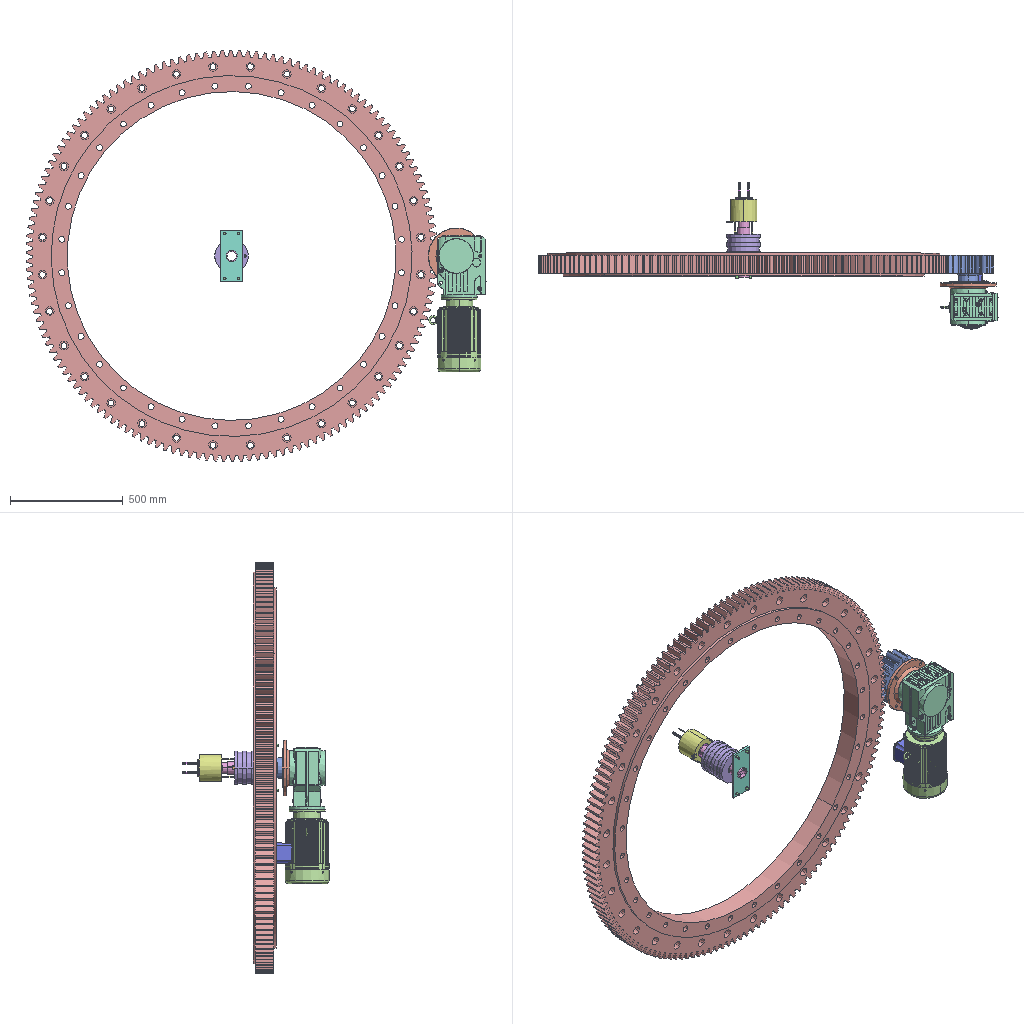Assembly | SolidWorks | 12 different items | 21 placed | box 2040 x 648 x 1824 mm
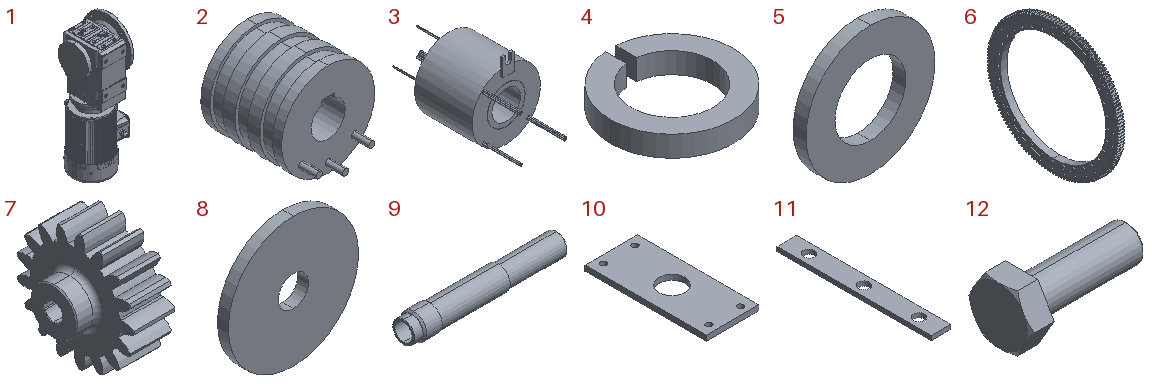Parts list (item | name | quantity | size | volume | features):
1 | (subassembly) | x1 | 274.5 x 257 x 638 mm | 13749904 mm3 | -
2 | - | x1 | 150 x 158 x 150 mm | 1845061 mm3 | features ICE 2, Revolution 1
3 | - | x1 | 119 x 236.5 x 137.5 mm | 931913 mm3 | features MBimport 1
4 | - | x4 | 15.372 x 15.344 x 2.6 mm | 261.313 mm3 | features Extrusion 1
5 | - | x4 | 20 x 2 x 20 mm | 438.252 mm3 | features Revolution 1
6 | - | x1 | 102 x 1824 x 1824 mm | 72400415 mm3 | features ICE 4, SketchHole 4, CirPattern 1, Stock 1
7 | - | x1 | 122 x 226.585 x 227.513 mm | 2321218 mm3 | features Chamfer 4, ICE 2, Fillet 1, MoveFace 1, SketchHole 1, Stock 1
8 | - | x1 | 60 x 5 x 60 mm | 13367 mm3 | features Extrusion 1
9 | - | x1 | 355 x 60 x 60 mm | 349894 mm3 | features Chamfer 1, Fillet 1, Revolution 1
10 | - | x1 | 100 x 230 x 10 mm | 206564 mm3 | features Extrusion 1
11 | - | x1 | 18 x 140 x 4 mm | 9138 mm3 | features Extrusion 1
12 | - | x4 | 36.4 x 18.475 x 16 mm | 3775 mm3 | features Chamfer 2, RevCut 2, Revolution 2, Extrusion 1, ICE 1
Mates (type | each side: item.copy, entity, surface, feature):
Concentric | 7.1 face cylinder Hole1 | 8.1 face cylinder Boss-Extrude1
Coincident | 6.1 face plane Cut-Extrude2 | 7.1 face plane Boss-Extrude1
Concentric | 3.1 face cylinder H50119-1810-2.stp<1> | 9.1 face cylinder Revolve3
DistanceDim | 9.1 face plane Revolve3 | 10.1 face plane Boss-Extrude1
Coincident | 2.1 face plane Revolve1 | 9.1 face plane Revolve3
Coincident | 3.1 face plane H50119-1810-2.stp<1> | 9.1 face plane Revolve3
Concentric | 3.1 face cylinder H50119-1810-2.stp<1> | 10.1 face cylinder Boss-Extrude1
Parallel | 3.1 face plane H50119-1810-2.stp<1> | 10.1 face plane Boss-Extrude1
Coincident | 10.1 edge | 5.1 edge
Coincident | 10.1 face plane Boss-Extrude1 | 5.1 face plane Base-Revolve
Concentric | 10.1 face cylinder Boss-Extrude1 | 4.1 face cylinder Extrude1
Coincident | 2.1 face plane Revolve1 | 11.1 face plane Boss-Extrude1
Coincident | 2.1 face plane Cut-Extrude1 | 11.1 face plane Boss-Extrude1 | 2 times
Parallel | 3.1 face plane H50119-1810-2.stp<1> | 11.1 face plane Boss-Extrude1
Concentric | 3.1 face cylinder H50119-1810-2.stp<1> | 2.1 face cylinder Cut-Extrude1
Coincident | 12.1 face plane Boss-Extrude1 | 4.1 face plane Extrude1
Coincident | 5.1 face plane Base-Revolve | 4.1 face plane Extrude1
Concentric | 12.2 face cylinder Revolve1 | 4.2 face cylinder Extrude1